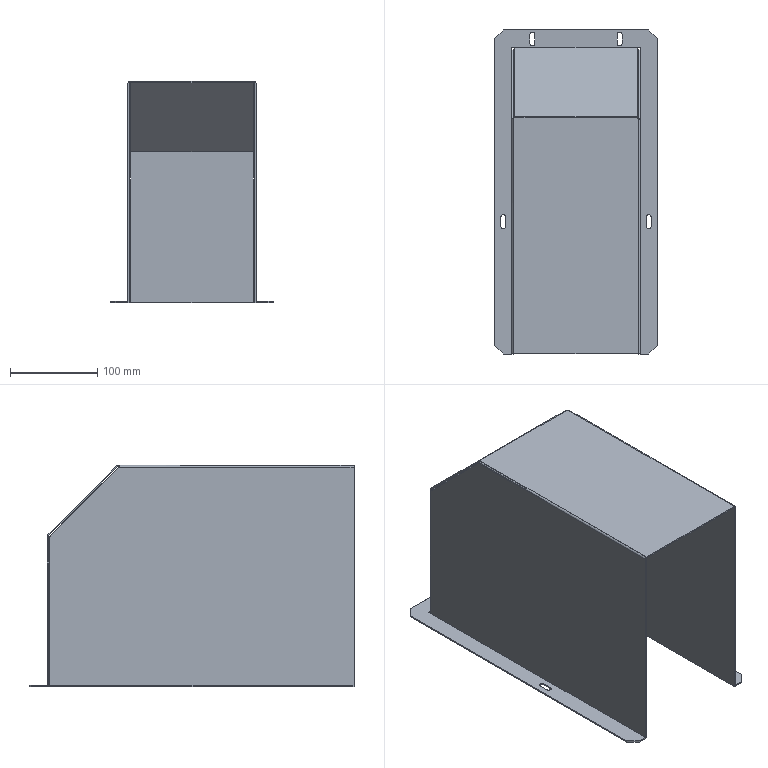Part | SolidWorks | features FlatPattern 2, SheetMetal 2, BreakCorner 1, Chamfer 1, Extrusion 1, HoleWzd 1, SMBaseFlange 1, SolidToSheetMetal 1 | 2 solids | 75 faces | box 187 x 372 x 254 mm | volume 400780 mm3 | plane 51 | cylinder 18 | spline 6 | commonest cylinder face diameters 5.8 x8 1.473 x6 4.473 x4